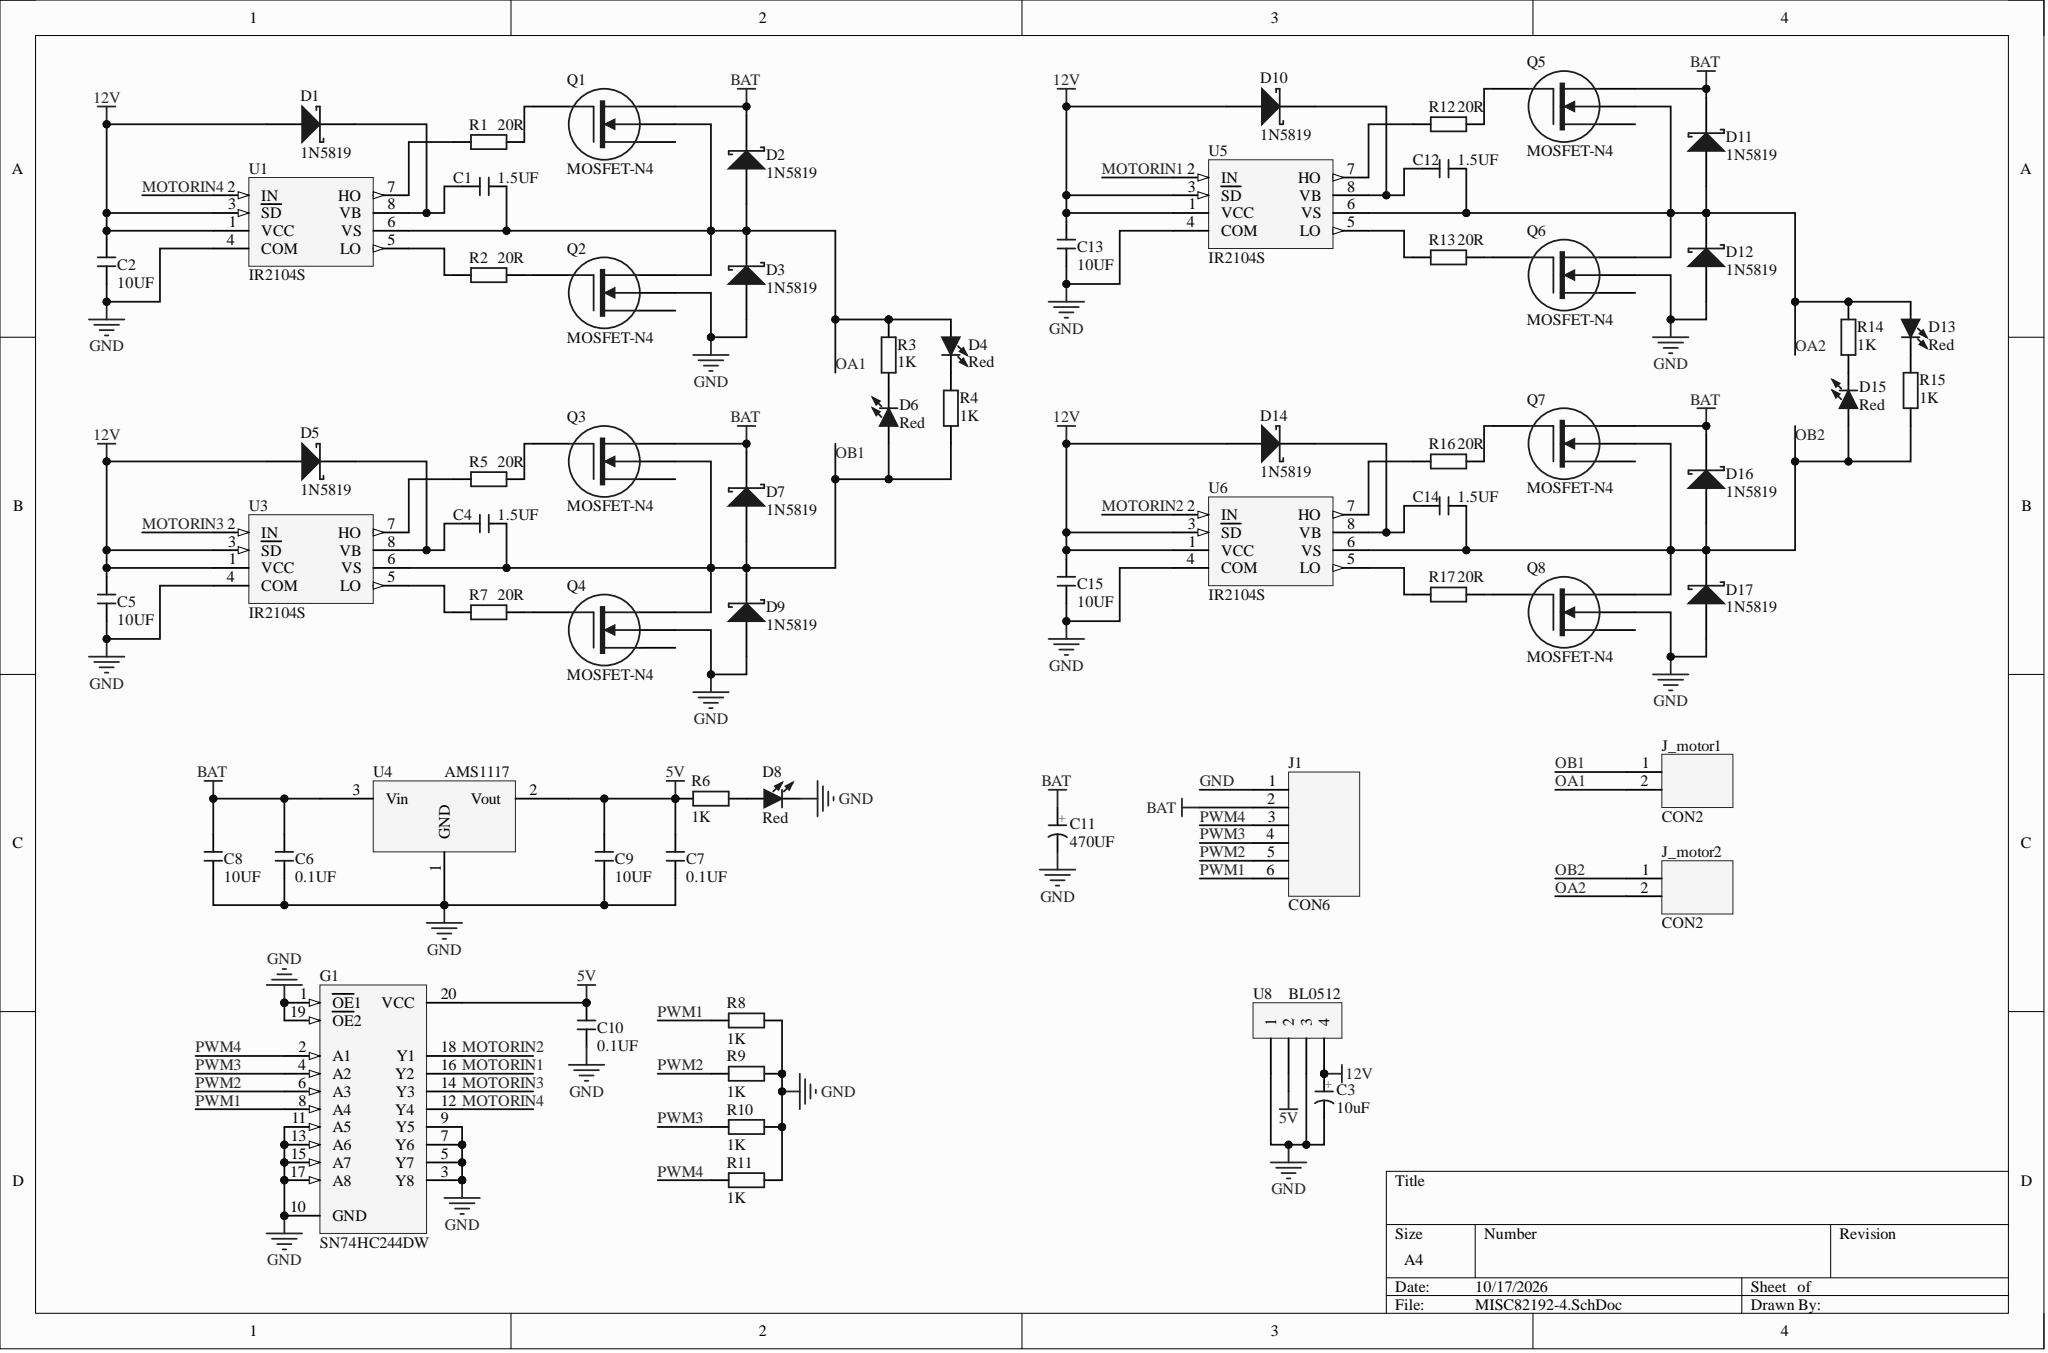Circuit board | Altium Designer | 67 parts | 41 nets
Bill of materials:
Comment,Description,Designator,Footprint,LibRef,Quantity
"1.5UF","SMD capacitor","C1, C4, C12, C14","C 0805_L","C","4"
"10UF","SMD capacitor, SMD solid-state capacitor","C2, C3, C5, C8, C9, C13, C15","C 0805_L","C, CS_SMD","7"
"0.1UF","SMD capacitor","C6, C7, C10","C 0805_L","C","3"
"470UF","SMD electrolytic capacitor","C11","CM A(3*5.4)","CE_SMD","1"
"1N5819","Schottky diode","D1, D2, D3, D5, D7, D9, D10, D11, D12, D14, D16, D17","SOD-323","1N5819","12"
"Red","SMD LED","D4, D6, D8, D13, D15","LED 0805G","LED-SMD","5"
"SN74HC244DW","Octal Buffer and Line Driver with 3-State Outputs","G1","DW020","SN74HC244DW","1"
"CON6","","J1","PH2.0-6P","PH2.0-6P","1"
"CON2","","J_motor1, J_motor2","PH2.0-2P","PH2.0-2P","2"
"MOSFET-N4","N-Channel MOSFET, Externally Terminated Substrate","Q1, Q2, Q3, Q4, Q5, Q6, Q7, Q8","TO252","MOSFET-N4","8"
"20R","SMD resistor","R1, R2, R5, R7, R12, R13, R16, R17","R 0805_L","R","8"
"1K","SMD resistor","R3, R4, R6, R8, R9, R10, R11, R14, R15","R 0805_L","R","9"
"IR2104S","High and Low Side Driver","U1, U3, U5, U6","SOP8","IR2104S","4"
"AMS1117","Three-terminal voltage regulator","U4","SOT223","AMS1117","1"
"BL0512","","U8","Fe-HDR1X4/2.54-S","Female HDR1X4","1"
Netlist (Protel format):
[
C1
C 0805_L
1.5UF



]
[
C2
C 0805_L
10UF



]
[
C3
C 0805_L
10uF



]
[
C4
C 0805_L
1.5UF



]
[
C5
C 0805_L
10UF



]
[
C6
C 0805_L
0.1UF



]
[
C7
C 0805_L
0.1UF



]
[
C8
C 0805_L
10UF



]
[
C9
C 0805_L
10UF



]
[
C10
C 0805_L
0.1UF



]
[
C11
CM A(3*5.4)
470UF



]
[
C12
C 0805_L
1.5UF



]
[
C13
C 0805_L
10UF



]
[
C14
C 0805_L
1.5UF



]
[
C15
C 0805_L
10UF



]
[
D1
SOD-323
1N5819



]
[
D2
SOD-323
1N5819



]
[
D3
SOD-323
1N5819



]
[
D4
LED 0805G
Red



]
[
D5
SOD-323
1N5819



]
[
D6
LED 0805G
Red



]
[
D7
SOD-323
1N5819



]
[
D8
LED 0805G
Red



]
[
D9
SOD-323
1N5819



]
[
D10
SOD-323
1N5819



]
[
D11
SOD-323
1N5819



]
[
D12
SOD-323
1N5819



]
[
D13
LED 0805G
Red



]
[
D14
SOD-323
1N5819



]
[
D15
LED 0805G
Red



]
[
D16
SOD-323
1N5819



]
[
D17
SOD-323
1N5819



]
[
G1
DW020
SN74HC244DW



]
[
J1
PH2.0-6P
CON6



]
[
J_motor1
PH2.0-2P
CON2



]
[
J_motor2
PH2.0-2P
CON2



]
[
Q1
TO252
MOSFET-N4



]
[
Q2
TO252
MOSFET-N4



]
[
Q3
TO252
MOSFET-N4



]
[
Q4
TO252
MOSFET-N4



]
[
Q5
TO252
MOSFET-N4



]
[
Q6
TO252
MOSFET-N4



]
[
Q7
TO252
MOSFET-N4



]
[
Q8
TO252
MOSFET-N4



]
[
R1
R 0805_L
20R



]
[
R2
R 0805_L
20R



]
[
R3
R 0805_L
1K



]
[
R4
R 0805_L
1K



]
[
R5
R 0805_L
20R



]
[
R6
R 0805_L
1K



]
[
R7
R 0805_L
20R



]
[
R8
R 0805_L
1K



]
[
R9
R 0805_L
1K



]
[
R10
R 0805_L
1K



]
[
R11
R 0805_L
1K



]
[
R12
R 0805_L
20R



]
[
R13
R 0805_L
20R



]
[
R14
R 0805_L
1K



]
[
R15
R 0805_L
1K



]
[
R16
R 0805_L
20R



]
[
R17
R 0805_L
20R



]
[
U1
SOP8
IR2104S



]
[
U3
SOP8
IR2104S



]
[
U4
SOT223
AMS1117



]
[
U5
SOP8
IR2104S



]
[
U6
SOP8
IR2104S



]
[
U8
Fe-HDR1X4/2.54-S
BL0512



]
(
PWM4
G1-2
J1-3
R11-1
)
(
PWM3
G1-4
J1-4
R10-1
)
(
PWM2
G1-6
J1-5
R9-1
)
(
PWM1
G1-8
J1-6
R8-1
)
(
OB2
C14-1
D15-1
D16-1
D17-2
J_motor2-1
Q7-3
Q8-4
R15-2
U6-6
)
(
OB1
C4-1
D6-1
D7-1
D9-2
J_motor1-1
Q3-3
Q4-4
R4-2
U3-6
)
(
OA2
C12-1
D11-1
D12-2
D13-1
J_motor2-2
Q5-3
Q6-4
R14-2
U5-6
)
(
OA1
C1-1
D2-1
D3-2
D4-1
J_motor1-2
Q1-3
Q2-4
R3-2
U1-6
)
(
NetR17_1
R17-1
U6-5
)
(
NetR16_1
R16-1
U6-7
)
(
NetR13_1
R13-1
U5-5
)
(
NetR12_1
R12-1
U5-7
)
(
NetR7_1
R7-1
U3-5
)
(
NetR5_1
R5-1
U3-7
)
(
NetR2_1
R2-1
U1-5
)
(
NetR1_1
R1-1
U1-7
)
(
NetQ8_1
Q8-1
R17-2
)
(
NetQ7_1
Q7-1
R16-2
)
(
NetQ6_1
Q6-1
R13-2
)
(
NetQ5_1
Q5-1
R12-2
)
(
NetQ4_1
Q4-1
R7-2
)
(
NetQ3_1
Q3-1
R5-2
)
(
NetQ2_1
Q2-1
R2-2
)
(
NetQ1_1
Q1-1
R1-2
)
(
NetD15_2
D15-2
R14-1
)
(
NetD13_2
D13-2
R15-1
)
(
NetD8_1
D8-1
R6-2
)
(
NetD6_2
D6-2
R3-1
)
(
NetD4_2
D4-2
R4-1
)
(
NetC14_2
C14-2
D14-2
U6-8
)
(
NetC12_2
C12-2
D10-2
U5-8
)
(
NetC4_2
C4-2
D5-2
U3-8
)
(
NetC1_2
C1-2
D1-2
U1-8
)
(
MOTORIN4
G1-12
U1-2
)
(
MOTORIN3
G1-14
U3-2
)
(
MOTORIN2
G1-18
U6-2
)
(
MOTORIN1
G1-16
U5-2
)
(
GND
C2-1
C3-2
C5-1
C6-1
C7-1
C8-1
C9-1
C10-1
C11-2
C13-1
C15-1
D3-1
D8-2
D9-1
D12-1
D17-1
G1-1
G1-3
G1-5
G1-7
G1-9
G1-10
G1-11
G1-13
G1-15
G1-17
G1-19
J1-1
Q2-3
Q4-3
Q6-3
Q8-3
R8-2
R9-2
R10-2
R11-2
U1-4
U3-4
U4-1
U5-4
U6-4
U8-1
U8-3
)
(
BAT
C6-2
C8-2
C11-1
D2-2
D7-2
D11-2
D16-2
J1-2
Q1-4
Q3-4
Q5-4
Q7-4
U4-3
)
(
12V
C2-2
C3-1
C5-2
C13-2
C15-2
D1-1
D5-1
D10-1
D14-1
U1-1
U1-3
U3-1
U3-3
U5-1
U5-3
U6-1
U6-3
U8-4
)
(
5V
C7-2
C9-2
C10-2
G1-20
R6-1
U4-2
U8-2
)